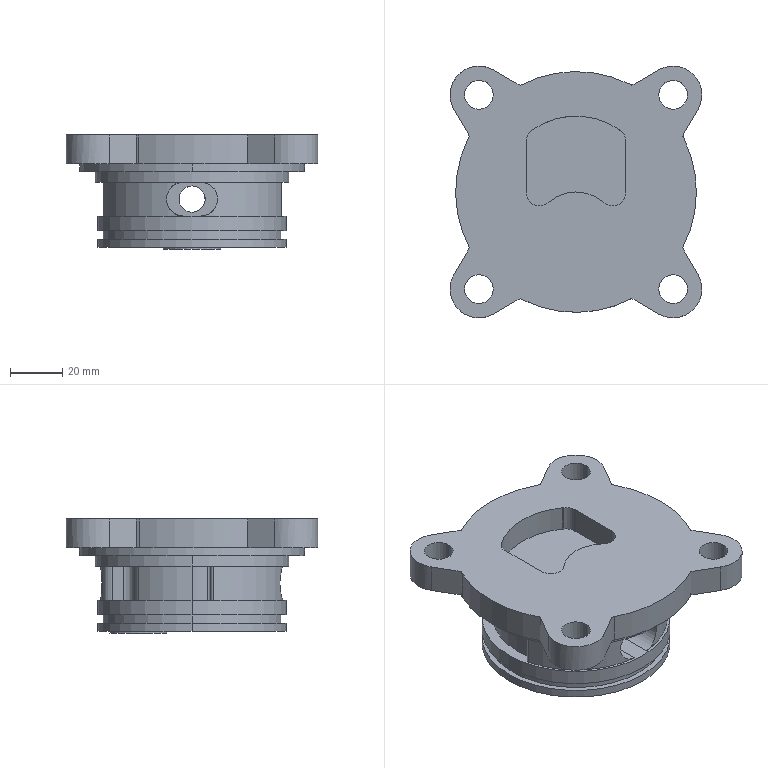Part | SolidWorks | features ICE 25, Fillet 7, HoleWzd 2, BaseBody 1 | 1 solid | 246 faces | box 96.247 x 96.248 x 43.6 mm | volume 156793 mm3 | cylinder 126 | plane 48 | torus 32 | spline 23 | cone 10 | sphere 7 | commonest cylinder face diameters 2 x35 10 x10 11 x8 92 x8 8 x6 22 x6